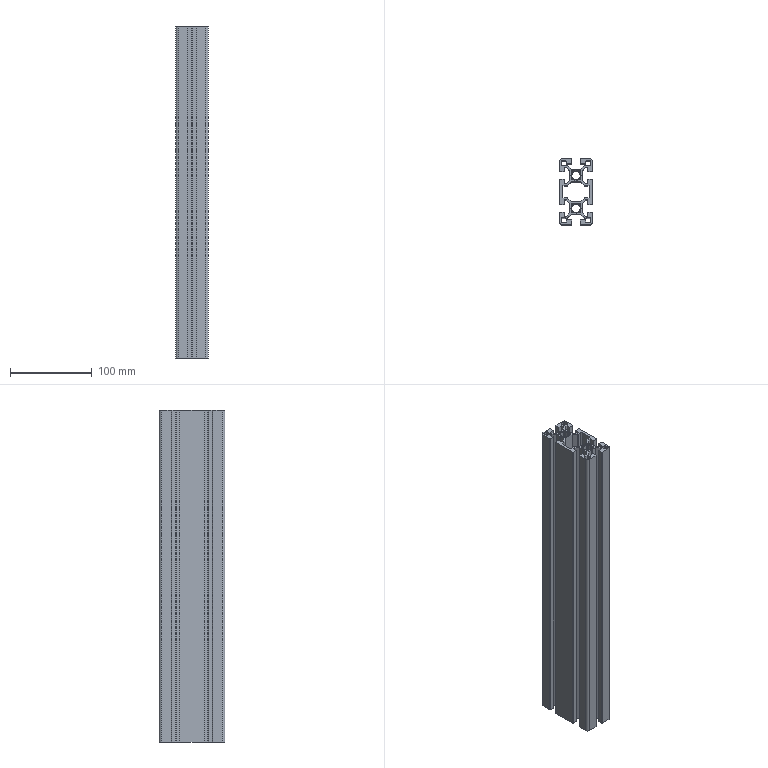Part | STEP file | 0245_023_HFS8-4080-405-TPW | 1 solid | 214 faces | box 40 x 80 x 405 mm | volume 451143 mm3 | plane 112 | cylinder 82 | cone 20 | commonest cylinder face diameters 2 x36 0.762 x20 0.6 x12 10.5 x10 6 x4